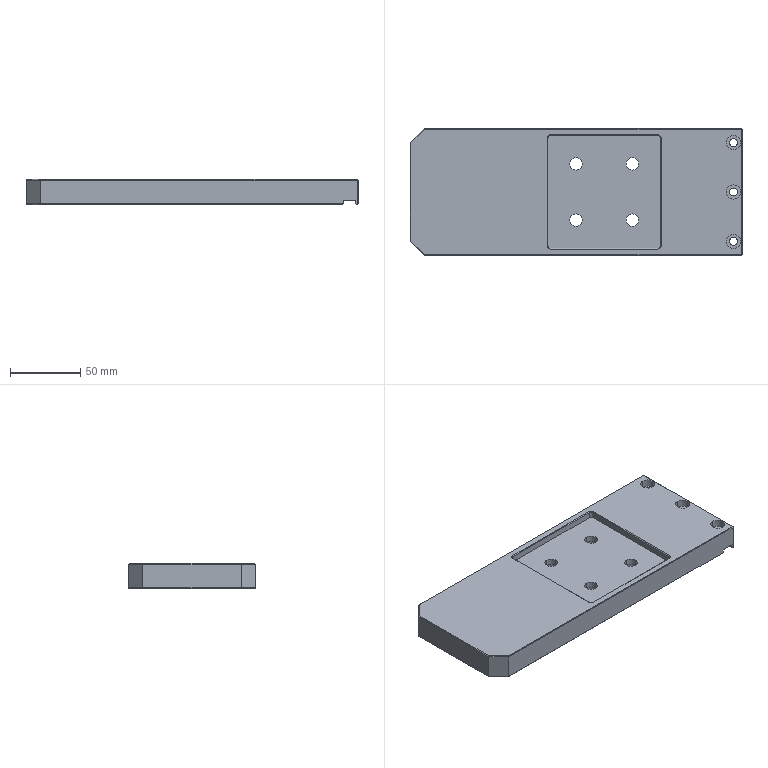Part | 1 solid | 82 faces | box 235.5 x 90 x 18 mm | volume 335919 mm3 | plane 46 | cylinder 32 | cone 4 | commonest cylinder face diameters 9 x8 15 x8 5.5 x6 10 x6 4 x4